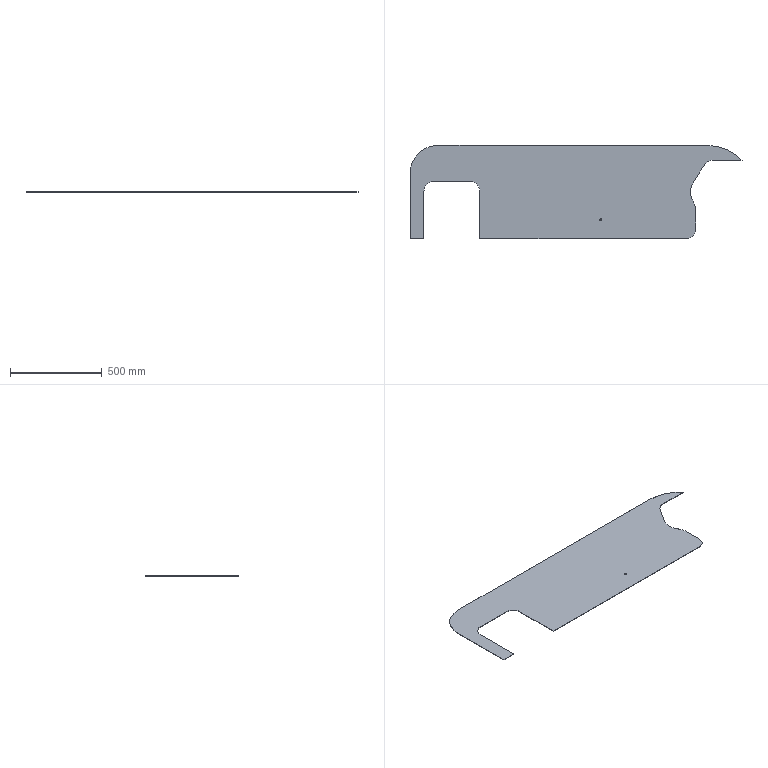Part | SolidWorks | features Extrusion 1 | 1 solid | 23 faces | box 1812 x 508 x 2 mm | volume 1419003 mm3 | plane 12 | cylinder 11 | commonest cylinder face diameters 101.6 x4 190.5 x3 11.176 x2 304.8 x1 508 x1
STEP:
#1=CARTESIAN_POINT('',(-589.788,-152.4,1.));
#2=VERTEX_POINT('',#1);
#3=CARTESIAN_POINT('',(-578.612,-152.4,1.));
#4=VERTEX_POINT('',#3);
#5=CARTESIAN_POINT('',(-584.2,-152.4,1.));
#6=DIRECTION('',(0.,0.,1.));
#7=DIRECTION('',(1.,0.,0.));
#8=AXIS2_PLACEMENT_3D('',#5,#6,#7);
#9=CIRCLE('',#8,5.588);
#10=EDGE_CURVE('',#2,#4,#9,.T.);
#11=ORIENTED_EDGE('',*,*,#10,.T.);
#12=CARTESIAN_POINT('',(-578.612,-152.4,-1.));
#13=VERTEX_POINT('',#12);
#14=CARTESIAN_POINT('',(-578.612,-152.4,1.));
#15=DIRECTION('',(0.,0.,-1.));
#16=VECTOR('',#15,1000.);
#17=LINE('',#14,#16);
#18=EDGE_CURVE('',#4,#13,#17,.T.);
#19=ORIENTED_EDGE('',*,*,#18,.T.);
#20=CARTESIAN_POINT('',(-589.788,-152.4,-1.));
#21=VERTEX_POINT('',#20);
#22=CARTESIAN_POINT('',(-584.2,-152.4,-1.));
#23=DIRECTION('',(0.,0.,1.));
#24=DIRECTION('',(1.,0.,0.));
#25=AXIS2_PLACEMENT_3D('',#22,#23,#24);
#26=CIRCLE('',#25,5.588);
#27=EDGE_CURVE('',#21,#13,#26,.T.);
#28=ORIENTED_EDGE('',*,*,#27,.F.);
#29=CARTESIAN_POINT('',(-589.788,-152.4,1.));
#30=DIRECTION('',(0.,0.,-1.));
#31=VECTOR('',#30,1000.);
#32=LINE('',#29,#31);
#33=EDGE_CURVE('',#2,#21,#32,.T.);
#34=ORIENTED_EDGE('',*,*,#33,.F.);
#35=EDGE_LOOP('',(#11,#19,#28,#34));
#36=FACE_OUTER_BOUND('',#35,.T.);
#37=CARTESIAN_POINT('',(-584.2,-152.4,1.));
#38=DIRECTION('',(0.,0.,-1.));
#39=DIRECTION('',(-1.,0.,0.));
#40=AXIS2_PLACEMENT_3D('',#37,#38,#39);
#41=CYLINDRICAL_SURFACE('',#40,5.588);
#42=ADVANCED_FACE('',(#36),#41,.F.);
#43=CARTESIAN_POINT('',(-95.25,0.,1.));
#44=VERTEX_POINT('',#43);
#45=CARTESIAN_POINT('',(-80.172,51.429,1.));
#46=VERTEX_POINT('',#45);
#47=CARTESIAN_POINT('',(0.,0.,1.));
#48=DIRECTION('',(0.,0.,-1.));
#49=DIRECTION('',(1.,0.,0.));
#50=AXIS2_PLACEMENT_3D('',#47,#48,#49);
#51=CIRCLE('',#50,95.25);
#52=EDGE_CURVE('',#44,#46,#51,.T.);
#53=ORIENTED_EDGE('',*,*,#52,.F.);
#54=CARTESIAN_POINT('',(-95.25,0.,-1.));
#55=VERTEX_POINT('',#54);
#56=CARTESIAN_POINT('',(-95.25,0.,1.));
#57=DIRECTION('',(0.,0.,-1.));
#58=VECTOR('',#57,1000.);
#59=LINE('',#56,#58);
#60=EDGE_CURVE('',#44,#55,#59,.T.);
#61=ORIENTED_EDGE('',*,*,#60,.T.);
#62=CARTESIAN_POINT('',(-80.172,51.429,-1.));
#63=VERTEX_POINT('',#62);
#64=CARTESIAN_POINT('',(0.,0.,-1.));
#65=DIRECTION('',(0.,0.,-1.));
#66=DIRECTION('',(1.,0.,0.));
#67=AXIS2_PLACEMENT_3D('',#64,#65,#66);
#68=CIRCLE('',#67,95.25);
#69=EDGE_CURVE('',#55,#63,#68,.T.);
#70=ORIENTED_EDGE('',*,*,#69,.T.);
#71=CARTESIAN_POINT('',(-80.172,51.429,1.));
#72=DIRECTION('',(0.,0.,-1.));
#73=VECTOR('',#72,1000.);
#74=LINE('',#71,#73);
#75=EDGE_CURVE('',#46,#63,#74,.T.);
#76=ORIENTED_EDGE('',*,*,#75,.F.);
#77=EDGE_LOOP('',(#53,#61,#70,#76));
#78=FACE_OUTER_BOUND('',#77,.T.);
#79=CARTESIAN_POINT('',(0.,0.,1.));
#80=DIRECTION('',(0.,0.,-1.));
#81=DIRECTION('',(-1.,0.,0.));
#82=AXIS2_PLACEMENT_3D('',#79,#80,#81);
#83=CYLINDRICAL_SURFACE('',#82,95.25);
#84=ADVANCED_FACE('',(#78),#83,.F.);
#85=CARTESIAN_POINT('',(-66.04,-101.37,1.));
#86=VERTEX_POINT('',#85);
#87=CARTESIAN_POINT('',(-80.645,-50.685,1.));
#88=VERTEX_POINT('',#87);
#89=CARTESIAN_POINT('',(-161.29,-101.37,1.));
#90=DIRECTION('',(0.,0.,1.));
#91=DIRECTION('',(1.,0.,0.));
#92=AXIS2_PLACEMENT_3D('',#89,#90,#91);
#93=CIRCLE('',#92,95.25);
#94=EDGE_CURVE('',#86,#88,#93,.T.);
#95=ORIENTED_EDGE('',*,*,#94,.T.);
#96=CARTESIAN_POINT('',(0.,0.,1.));
#97=DIRECTION('',(0.,0.,-1.));
#98=DIRECTION('',(1.,0.,0.));
#99=AXIS2_PLACEMENT_3D('',#96,#97,#98);
#100=CIRCLE('',#99,95.25);
#101=EDGE_CURVE('',#88,#44,#100,.T.);
#102=ORIENTED_EDGE('',*,*,#101,.T.);
#103=ORIENTED_EDGE('',*,*,#52,.T.);
#104=CARTESIAN_POINT('',(-17.359,149.349,1.));
#105=VERTEX_POINT('',#104);
#106=CARTESIAN_POINT('',(-17.359,149.349,1.));
#107=DIRECTION('',(0.5399,0.8417,0.));
#108=VECTOR('',#107,1000.);
#109=LINE('',#106,#108);
#110=EDGE_CURVE('',#46,#105,#109,.T.);
#111=ORIENTED_EDGE('',*,*,#110,.T.);
#112=CARTESIAN_POINT('',(25.4,172.72,1.));
#113=VERTEX_POINT('',#112);
#114=CARTESIAN_POINT('',(25.4,121.92,1.));
#115=DIRECTION('',(0.,0.,-1.));
#116=DIRECTION('',(1.,0.,0.));
#117=AXIS2_PLACEMENT_3D('',#114,#115,#116);
#118=CIRCLE('',#117,50.8);
#119=EDGE_CURVE('',#105,#113,#118,.T.);
#120=ORIENTED_EDGE('',*,*,#119,.T.);
#121=CARTESIAN_POINT('',(186.236,172.72,1.));
#122=VERTEX_POINT('',#121);
#123=CARTESIAN_POINT('',(186.236,172.72,1.));
#124=DIRECTION('',(1.,0.,0.));
#125=VECTOR('',#124,1000.);
#126=LINE('',#123,#125);
#127=EDGE_CURVE('',#113,#122,#126,.T.);
#128=ORIENTED_EDGE('',*,*,#127,.T.);
#129=CARTESIAN_POINT('',(0.,254.,1.));
#130=VERTEX_POINT('',#129);
#131=CARTESIAN_POINT('',(0.,0.,1.));
#132=DIRECTION('',(0.,0.,1.));
#133=DIRECTION('',(1.,0.,0.));
#134=AXIS2_PLACEMENT_3D('',#131,#132,#133);
#135=CIRCLE('',#134,254.);
#136=EDGE_CURVE('',#122,#130,#135,.T.);
#137=ORIENTED_EDGE('',*,*,#136,.T.);
#138=CARTESIAN_POINT('',(-1473.2,254.,1.));
#139=VERTEX_POINT('',#138);
#140=CARTESIAN_POINT('',(0.,254.,1.));
#141=DIRECTION('',(-1.,0.,0.));
#142=VECTOR('',#141,1000.);
#143=LINE('',#140,#142);
#144=EDGE_CURVE('',#130,#139,#143,.T.);
#145=ORIENTED_EDGE('',*,*,#144,.T.);
#146=CARTESIAN_POINT('',(-1625.6,101.6,1.));
#147=VERTEX_POINT('',#146);
#148=CARTESIAN_POINT('',(-1473.2,101.6,1.));
#149=DIRECTION('',(0.,0.,1.));
#150=DIRECTION('',(1.,0.,0.));
#151=AXIS2_PLACEMENT_3D('',#148,#149,#150);
#152=CIRCLE('',#151,152.4);
#153=EDGE_CURVE('',#139,#147,#152,.T.);
#154=ORIENTED_EDGE('',*,*,#153,.T.);
#155=CARTESIAN_POINT('',(-1625.6,-254.,1.));
#156=VERTEX_POINT('',#155);
#157=CARTESIAN_POINT('',(-1625.6,101.6,1.));
#158=DIRECTION('',(0.,-1.,0.));
#159=VECTOR('',#158,1000.);
#160=LINE('',#157,#159);
#161=EDGE_CURVE('',#147,#156,#160,.T.);
#162=ORIENTED_EDGE('',*,*,#161,.T.);
#163=CARTESIAN_POINT('',(-1549.4,-254.,1.));
#164=VERTEX_POINT('',#163);
#165=CARTESIAN_POINT('',(-1549.4,-254.,1.));
#166=DIRECTION('',(1.,0.,0.));
#167=VECTOR('',#166,1000.);
#168=LINE('',#165,#167);
#169=EDGE_CURVE('',#156,#164,#168,.T.);
#170=ORIENTED_EDGE('',*,*,#169,.T.);
#171=CARTESIAN_POINT('',(-1549.4,5.08,1.));
#172=VERTEX_POINT('',#171);
#173=CARTESIAN_POINT('',(-1549.4,-254.,1.));
#174=DIRECTION('',(0.,1.,0.));
#175=VECTOR('',#174,1000.);
#176=LINE('',#173,#175);
#177=EDGE_CURVE('',#164,#172,#176,.T.);
#178=ORIENTED_EDGE('',*,*,#177,.T.);
#179=CARTESIAN_POINT('',(-1498.6,55.88,1.));
#180=VERTEX_POINT('',#179);
#181=CARTESIAN_POINT('',(-1498.6,5.08,1.));
#182=DIRECTION('',(0.,0.,-1.));
#183=DIRECTION('',(-1.,0.,0.));
#184=AXIS2_PLACEMENT_3D('',#181,#182,#183);
#185=CIRCLE('',#184,50.8);
#186=EDGE_CURVE('',#172,#180,#185,.T.);
#187=ORIENTED_EDGE('',*,*,#186,.T.);
#188=CARTESIAN_POINT('',(-1295.4,55.88,1.));
#189=VERTEX_POINT('',#188);
#190=CARTESIAN_POINT('',(-1498.6,55.88,1.));
#191=DIRECTION('',(1.,0.,0.));
#192=VECTOR('',#191,1000.);
#193=LINE('',#190,#192);
#194=EDGE_CURVE('',#180,#189,#193,.T.);
#195=ORIENTED_EDGE('',*,*,#194,.T.);
#196=CARTESIAN_POINT('',(-1244.6,5.08,1.));
#197=VERTEX_POINT('',#196);
#198=CARTESIAN_POINT('',(-1295.4,5.08,1.));
#199=DIRECTION('',(0.,0.,-1.));
#200=DIRECTION('',(-1.,0.,0.));
#201=AXIS2_PLACEMENT_3D('',#198,#199,#200);
#202=CIRCLE('',#201,50.8);
#203=EDGE_CURVE('',#189,#197,#202,.T.);
#204=ORIENTED_EDGE('',*,*,#203,.T.);
#205=CARTESIAN_POINT('',(-1244.6,-254.,1.));
#206=VERTEX_POINT('',#205);
#207=CARTESIAN_POINT('',(-1244.6,5.08,1.));
#208=DIRECTION('',(0.,-1.,0.));
#209=VECTOR('',#208,1000.);
#210=LINE('',#207,#209);
#211=EDGE_CURVE('',#197,#206,#210,.T.);
#212=ORIENTED_EDGE('',*,*,#211,.T.);
#213=CARTESIAN_POINT('',(-116.84,-254.,1.));
#214=VERTEX_POINT('',#213);
#215=CARTESIAN_POINT('',(-116.84,-254.,1.));
#216=DIRECTION('',(1.,0.,0.));
#217=VECTOR('',#216,1000.);
#218=LINE('',#215,#217);
#219=EDGE_CURVE('',#206,#214,#218,.T.);
#220=ORIENTED_EDGE('',*,*,#219,.T.);
#221=CARTESIAN_POINT('',(-66.04,-203.2,1.));
#222=VERTEX_POINT('',#221);
#223=CARTESIAN_POINT('',(-116.84,-203.2,1.));
#224=DIRECTION('',(0.,0.,1.));
#225=DIRECTION('',(-1.,0.,0.));
#226=AXIS2_PLACEMENT_3D('',#223,#224,#225);
#227=CIRCLE('',#226,50.8);
#228=EDGE_CURVE('',#214,#222,#227,.T.);
#229=ORIENTED_EDGE('',*,*,#228,.T.);
#230=CARTESIAN_POINT('',(-66.04,-101.37,1.));
#231=DIRECTION('',(0.,1.,0.));
#232=VECTOR('',#231,1000.);
#233=LINE('',#230,#232);
#234=EDGE_CURVE('',#222,#86,#233,.T.);
#235=ORIENTED_EDGE('',*,*,#234,.T.);
#236=EDGE_LOOP('',(#95,#102,#103,#111,#120,#128,#137,#145,#154,#162,#170,#178,#187,#195,#204,#212,#220,#229,#235));
#237=FACE_OUTER_BOUND('',#236,.T.);
#238=ORIENTED_EDGE('',*,*,#10,.F.);
#239=CARTESIAN_POINT('',(-584.2,-152.4,1.));
#240=DIRECTION('',(0.,0.,1.));
#241=DIRECTION('',(1.,0.,0.));
#242=AXIS2_PLACEMENT_3D('',#239,#240,#241);
#243=CIRCLE('',#242,5.588);
#244=EDGE_CURVE('',#4,#2,#243,.T.);
#245=ORIENTED_EDGE('',*,*,#244,.F.);
#246=EDGE_LOOP('',(#238,#245));
#247=FACE_BOUND('',#246,.T.);
#248=CARTESIAN_POINT('',(-161.29,-101.37,1.));
#249=DIRECTION('',(0.,0.,1.));
#250=DIRECTION('',(1.,0.,0.));
#251=AXIS2_PLACEMENT_3D('',#248,#249,#250);
#252=PLANE('',#251);
#253=ADVANCED_FACE('',(#237,#247),#252,.T.);
#254=CARTESIAN_POINT('',(-66.04,-101.37,-1.));
#255=VERTEX_POINT('',#254);
#256=CARTESIAN_POINT('',(-80.645,-50.685,-1.));
#257=VERTEX_POINT('',#256);
#258=CARTESIAN_POINT('',(-161.29,-101.37,-1.));
#259=DIRECTION('',(0.,0.,1.));
#260=DIRECTION('',(1.,0.,0.));
#261=AXIS2_PLACEMENT_3D('',#258,#259,#260);
#262=CIRCLE('',#261,95.25);
#263=EDGE_CURVE('',#255,#257,#262,.T.);
#264=ORIENTED_EDGE('',*,*,#263,.F.);
#265=CARTESIAN_POINT('',(-66.04,-203.2,-1.));
#266=VERTEX_POINT('',#265);
#267=CARTESIAN_POINT('',(-66.04,-101.37,-1.));
#268=DIRECTION('',(0.,1.,0.));
#269=VECTOR('',#268,1000.);
#270=LINE('',#267,#269);
#271=EDGE_CURVE('',#266,#255,#270,.T.);
#272=ORIENTED_EDGE('',*,*,#271,.F.);
#273=CARTESIAN_POINT('',(-116.84,-254.,-1.));
#274=VERTEX_POINT('',#273);
#275=CARTESIAN_POINT('',(-116.84,-203.2,-1.));
#276=DIRECTION('',(0.,0.,1.));
#277=DIRECTION('',(-1.,0.,0.));
#278=AXIS2_PLACEMENT_3D('',#275,#276,#277);
#279=CIRCLE('',#278,50.8);
#280=EDGE_CURVE('',#274,#266,#279,.T.);
#281=ORIENTED_EDGE('',*,*,#280,.F.);
#282=CARTESIAN_POINT('',(-1244.6,-254.,-1.));
#283=VERTEX_POINT('',#282);
#284=CARTESIAN_POINT('',(-116.84,-254.,-1.));
#285=DIRECTION('',(1.,0.,0.));
#286=VECTOR('',#285,1000.);
#287=LINE('',#284,#286);
#288=EDGE_CURVE('',#283,#274,#287,.T.);
#289=ORIENTED_EDGE('',*,*,#288,.F.);
#290=CARTESIAN_POINT('',(-1244.6,5.08,-1.));
#291=VERTEX_POINT('',#290);
#292=CARTESIAN_POINT('',(-1244.6,5.08,-1.));
#293=DIRECTION('',(0.,-1.,0.));
#294=VECTOR('',#293,1000.);
#295=LINE('',#292,#294);
#296=EDGE_CURVE('',#291,#283,#295,.T.);
#297=ORIENTED_EDGE('',*,*,#296,.F.);
#298=CARTESIAN_POINT('',(-1295.4,55.88,-1.));
#299=VERTEX_POINT('',#298);
#300=CARTESIAN_POINT('',(-1295.4,5.08,-1.));
#301=DIRECTION('',(0.,0.,-1.));
#302=DIRECTION('',(-1.,0.,0.));
#303=AXIS2_PLACEMENT_3D('',#300,#301,#302);
#304=CIRCLE('',#303,50.8);
#305=EDGE_CURVE('',#299,#291,#304,.T.);
#306=ORIENTED_EDGE('',*,*,#305,.F.);
#307=CARTESIAN_POINT('',(-1498.6,55.88,-1.));
#308=VERTEX_POINT('',#307);
#309=CARTESIAN_POINT('',(-1498.6,55.88,-1.));
#310=DIRECTION('',(1.,0.,0.));
#311=VECTOR('',#310,1000.);
#312=LINE('',#309,#311);
#313=EDGE_CURVE('',#308,#299,#312,.T.);
#314=ORIENTED_EDGE('',*,*,#313,.F.);
#315=CARTESIAN_POINT('',(-1549.4,5.08,-1.));
#316=VERTEX_POINT('',#315);
#317=CARTESIAN_POINT('',(-1498.6,5.08,-1.));
#318=DIRECTION('',(0.,0.,-1.));
#319=DIRECTION('',(-1.,0.,0.));
#320=AXIS2_PLACEMENT_3D('',#317,#318,#319);
#321=CIRCLE('',#320,50.8);
#322=EDGE_CURVE('',#316,#308,#321,.T.);
#323=ORIENTED_EDGE('',*,*,#322,.F.);
#324=CARTESIAN_POINT('',(-1549.4,-254.,-1.));
#325=VERTEX_POINT('',#324);
#326=CARTESIAN_POINT('',(-1549.4,-254.,-1.));
#327=DIRECTION('',(0.,1.,0.));
#328=VECTOR('',#327,1000.);
#329=LINE('',#326,#328);
#330=EDGE_CURVE('',#325,#316,#329,.T.);
#331=ORIENTED_EDGE('',*,*,#330,.F.);
#332=CARTESIAN_POINT('',(-1625.6,-254.,-1.));
#333=VERTEX_POINT('',#332);
#334=CARTESIAN_POINT('',(-1549.4,-254.,-1.));
#335=DIRECTION('',(1.,0.,0.));
#336=VECTOR('',#335,1000.);
#337=LINE('',#334,#336);
#338=EDGE_CURVE('',#333,#325,#337,.T.);
#339=ORIENTED_EDGE('',*,*,#338,.F.);
#340=CARTESIAN_POINT('',(-1625.6,101.6,-1.));
#341=VERTEX_POINT('',#340);
#342=CARTESIAN_POINT('',(-1625.6,101.6,-1.));
#343=DIRECTION('',(0.,-1.,0.));
#344=VECTOR('',#343,1000.);
#345=LINE('',#342,#344);
#346=EDGE_CURVE('',#341,#333,#345,.T.);
#347=ORIENTED_EDGE('',*,*,#346,.F.);
#348=CARTESIAN_POINT('',(-1473.2,254.,-1.));
#349=VERTEX_POINT('',#348);
#350=CARTESIAN_POINT('',(-1473.2,101.6,-1.));
#351=DIRECTION('',(0.,0.,1.));
#352=DIRECTION('',(1.,0.,0.));
#353=AXIS2_PLACEMENT_3D('',#350,#351,#352);
#354=CIRCLE('',#353,152.4);
#355=EDGE_CURVE('',#349,#341,#354,.T.);
#356=ORIENTED_EDGE('',*,*,#355,.F.);
#357=CARTESIAN_POINT('',(0.,254.,-1.));
#358=VERTEX_POINT('',#357);
#359=CARTESIAN_POINT('',(0.,254.,-1.));
#360=DIRECTION('',(-1.,0.,0.));
#361=VECTOR('',#360,1000.);
#362=LINE('',#359,#361);
#363=EDGE_CURVE('',#358,#349,#362,.T.);
#364=ORIENTED_EDGE('',*,*,#363,.F.);
#365=CARTESIAN_POINT('',(186.236,172.72,-1.));
#366=VERTEX_POINT('',#365);
#367=CARTESIAN_POINT('',(0.,0.,-1.));
#368=DIRECTION('',(0.,0.,1.));
#369=DIRECTION('',(1.,0.,0.));
#370=AXIS2_PLACEMENT_3D('',#367,#368,#369);
#371=CIRCLE('',#370,254.);
#372=EDGE_CURVE('',#366,#358,#371,.T.);
#373=ORIENTED_EDGE('',*,*,#372,.F.);
#374=CARTESIAN_POINT('',(25.4,172.72,-1.));
#375=VERTEX_POINT('',#374);
#376=CARTESIAN_POINT('',(186.236,172.72,-1.));
#377=DIRECTION('',(1.,0.,0.));
#378=VECTOR('',#377,1000.);
#379=LINE('',#376,#378);
#380=EDGE_CURVE('',#375,#366,#379,.T.);
#381=ORIENTED_EDGE('',*,*,#380,.F.);
#382=CARTESIAN_POINT('',(-17.359,149.349,-1.));
#383=VERTEX_POINT('',#382);
#384=CARTESIAN_POINT('',(25.4,121.92,-1.));
#385=DIRECTION('',(0.,0.,-1.));
#386=DIRECTION('',(1.,0.,0.));
#387=AXIS2_PLACEMENT_3D('',#384,#385,#386);
#388=CIRCLE('',#387,50.8);
#389=EDGE_CURVE('',#383,#375,#388,.T.);
#390=ORIENTED_EDGE('',*,*,#389,.F.);
#391=CARTESIAN_POINT('',(-17.359,149.349,-1.));
#392=DIRECTION('',(0.5399,0.8417,0.));
#393=VECTOR('',#392,1000.);
#394=LINE('',#391,#393);
#395=EDGE_CURVE('',#63,#383,#394,.T.);
#396=ORIENTED_EDGE('',*,*,#395,.F.);
#397=ORIENTED_EDGE('',*,*,#69,.F.);
#398=CARTESIAN_POINT('',(0.,0.,-1.));
#399=DIRECTION('',(0.,0.,-1.));
#400=DIRECTION('',(1.,0.,0.));
#401=AXIS2_PLACEMENT_3D('',#398,#399,#400);
#402=CIRCLE('',#401,95.25);
#403=EDGE_CURVE('',#257,#55,#402,.T.);
#404=ORIENTED_EDGE('',*,*,#403,.F.);
#405=EDGE_LOOP('',(#264,#272,#281,#289,#297,#306,#314,#323,#331,#339,#347,#356,#364,#373,#381,#390,#396,#397,#404));
#406=FACE_OUTER_BOUND('',#405,.T.);
#407=ORIENTED_EDGE('',*,*,#27,.T.);
#408=CARTESIAN_POINT('',(-584.2,-152.4,-1.));
#409=DIRECTION('',(0.,0.,1.));
#410=DIRECTION('',(1.,0.,0.));
#411=AXIS2_PLACEMENT_3D('',#408,#409,#410);
#412=CIRCLE('',#411,5.588);
#413=EDGE_CURVE('',#13,#21,#412,.T.);
#414=ORIENTED_EDGE('',*,*,#413,.T.);
#415=EDGE_LOOP('',(#407,#414));
#416=FACE_BOUND('',#415,.T.);
#417=CARTESIAN_POINT('',(-161.29,-101.37,-1.));
#418=DIRECTION('',(0.,0.,1.));
#419=DIRECTION('',(1.,0.,0.));
#420=AXIS2_PLACEMENT_3D('',#417,#418,#419);
#421=PLANE('',#420);
#422=ADVANCED_FACE('',(#406,#416),#421,.F.);
#423=ORIENTED_EDGE('',*,*,#263,.T.);
#424=CARTESIAN_POINT('',(-80.645,-50.685,1.));
#425=DIRECTION('',(0.,0.,-1.));
#426=VECTOR('',#425,1000.);
#427=LINE('',#424,#426);
#428=EDGE_CURVE('',#88,#257,#427,.T.);
#429=ORIENTED_EDGE('',*,*,#428,.F.);
#430=ORIENTED_EDGE('',*,*,#94,.F.);
#431=CARTESIAN_POINT('',(-66.04,-101.37,1.));
#432=DIRECTION('',(0.,0.,-1.));
#433=VECTOR('',#432,1000.);
#434=LINE('',#431,#433);
#435=EDGE_CURVE('',#86,#255,#434,.T.);
#436=ORIENTED_EDGE('',*,*,#435,.T.);
#437=EDGE_LOOP('',(#423,#429,#430,#436));
#438=FACE_OUTER_BOUND('',#437,.T.);
#439=CARTESIAN_POINT('',(-161.29,-101.37,1.));
#440=DIRECTION('',(0.,0.,-1.));
#441=DIRECTION('',(-1.,0.,0.));
#442=AXIS2_PLACEMENT_3D('',#439,#440,#441);
#443=CYLINDRICAL_SURFACE('',#442,95.25);
#444=ADVANCED_FACE('',(#438),#443,.T.);
#445=ORIENTED_EDGE('',*,*,#60,.F.);
#446=ORIENTED_EDGE('',*,*,#101,.F.);
#447=ORIENTED_EDGE('',*,*,#428,.T.);
#448=ORIENTED_EDGE('',*,*,#403,.T.);
#449=EDGE_LOOP('',(#445,#446,#447,#448));
#450=FACE_OUTER_BOUND('',#449,.T.);
#451=CARTESIAN_POINT('',(0.,0.,1.));
#452=DIRECTION('',(0.,0.,-1.));
#453=DIRECTION('',(-1.,0.,0.));
#454=AXIS2_PLACEMENT_3D('',#451,#452,#453);
#455=CYLINDRICAL_SURFACE('',#454,95.25);
#456=ADVANCED_FACE('',(#450),#455,.F.);
#457=ORIENTED_EDGE('',*,*,#395,.T.);
#458=CARTESIAN_POINT('',(-17.359,149.349,1.));
#459=DIRECTION('',(0.,0.,-1.));
#460=VECTOR('',#459,1000.);
#461=LINE('',#458,#460);
#462=EDGE_CURVE('',#105,#383,#461,.T.);
#463=ORIENTED_EDGE('',*,*,#462,.F.);
#464=ORIENTED_EDGE('',*,*,#110,.F.);
#465=ORIENTED_EDGE('',*,*,#75,.T.);
#466=EDGE_LOOP('',(#457,#463,#464,#465));
#467=FACE_OUTER_BOUND('',#466,.T.);
#468=CARTESIAN_POINT('',(-17.359,149.349,1.));
#469=DIRECTION('',(-0.8417,0.5399,0.));
#470=DIRECTION('',(-0.5399,-0.8417,0.));
#471=AXIS2_PLACEMENT_3D('',#468,#469,#470);
#472=PLANE('',#471);
#473=ADVANCED_FACE('',(#467),#472,.F.);
#474=ORIENTED_EDGE('',*,*,#389,.T.);
#475=CARTESIAN_POINT('',(25.4,172.72,1.));
#476=DIRECTION('',(0.,0.,-1.));
#477=VECTOR('',#476,1000.);
#478=LINE('',#475,#477);
#479=EDGE_CURVE('',#113,#375,#478,.T.);
#480=ORIENTED_EDGE('',*,*,#479,.F.);
#481=ORIENTED_EDGE('',*,*,#119,.F.);
#482=ORIENTED_EDGE('',*,*,#462,.T.);
#483=EDGE_LOOP('',(#474,#480,#481,#482));
#484=FACE_OUTER_BOUND('',#483,.T.);
#485=CARTESIAN_POINT('',(25.4,121.92,1.));
#486=DIRECTION('',(0.,0.,-1.));
#487=DIRECTION('',(-1.,0.,0.));
#488=AXIS2_PLACEMENT_3D('',#485,#486,#487);
#489=CYLINDRICAL_SURFACE('',#488,50.8);
#490=ADVANCED_FACE('',(#484),#489,.F.);
#491=ORIENTED_EDGE('',*,*,#380,.T.);
#492=CARTESIAN_POINT('',(186.236,172.72,1.));
#493=DIRECTION('',(0.,0.,-1.));
#494=VECTOR('',#493,1000.);
#495=LINE('',#492,#494);
#496=EDGE_CURVE('',#122,#366,#495,.T.);
#497=ORIENTED_EDGE('',*,*,#496,.F.);
#498=ORIENTED_EDGE('',*,*,#127,.F.);
#499=ORIENTED_EDGE('',*,*,#479,.T.);
#500=EDGE_LOOP('',(#491,#497,#498,#499));
#501=FACE_OUTER_BOUND('',#500,.T.);
#502=CARTESIAN_POINT('',(186.236,172.72,1.));
#503=DIRECTION('',(0.,1.,0.));
#504=DIRECTION('',(-1.,0.,0.));
#505=AXIS2_PLACEMENT_3D('',#502,#503,#504);
#506=PLANE('',#505);
#507=ADVANCED_FACE('',(#501),#506,.F.);
#508=ORIENTED_EDGE('',*,*,#372,.T.);
#509=CARTESIAN_POINT('',(0.,254.,1.));
#510=DIRECTION('',(0.,0.,-1.));
#511=VECTOR('',#510,1000.);
#512=LINE('',#509,#511);
#513=EDGE_CURVE('',#130,#358,#512,.T.);
#514=ORIENTED_EDGE('',*,*,#513,.F.);
#515=ORIENTED_EDGE('',*,*,#136,.F.);
#516=ORIENTED_EDGE('',*,*,#496,.T.);
#517=EDGE_LOOP('',(#508,#514,#515,#516));
#518=FACE_OUTER_BOUND('',#517,.T.);
#519=CARTESIAN_POINT('',(0.,0.,1.));
#520=DIRECTION('',(0.,0.,-1.));
#521=DIRECTION('',(-1.,0.,0.));
#522=AXIS2_PLACEMENT_3D('',#519,#520,#521);
#523=CYLINDRICAL_SURFACE('',#522,254.);
#524=ADVANCED_FACE('',(#518),#523,.T.);
#525=ORIENTED_EDGE('',*,*,#363,.T.);
#526=CARTESIAN_POINT('',(-1473.2,254.,1.));
#527=DIRECTION('',(0.,0.,-1.));
#528=VECTOR('',#527,1000.);
#529=LINE('',#526,#528);
#530=EDGE_CURVE('',#139,#349,#529,.T.);
#531=ORIENTED_EDGE('',*,*,#530,.F.);
#532=ORIENTED_EDGE('',*,*,#144,.F.);
#533=ORIENTED_EDGE('',*,*,#513,.T.);
#534=EDGE_LOOP('',(#525,#531,#532,#533));
#535=FACE_OUTER_BOUND('',#534,.T.);
#536=CARTESIAN_POINT('',(0.,254.,1.));
#537=DIRECTION('',(0.,-1.,0.));
#538=DIRECTION('',(1.,0.,0.));
#539=AXIS2_PLACEMENT_3D('',#536,#537,#538);
#540=PLANE('',#539);
#541=ADVANCED_FACE('',(#535),#540,.F.);
#542=ORIENTED_EDGE('',*,*,#355,.T.);
#543=CARTESIAN_POINT('',(-1625.6,101.6,1.));
#544=DIRECTION('',(0.,0.,-1.));
#545=VECTOR('',#544,1000.);
#546=LINE('',#543,#545);
#547=EDGE_CURVE('',#147,#341,#546,.T.);
#548=ORIENTED_EDGE('',*,*,#547,.F.);
#549=ORIENTED_EDGE('',*,*,#153,.F.);
#550=ORIENTED_EDGE('',*,*,#530,.T.);
#551=EDGE_LOOP('',(#542,#548,#549,#550));
#552=FACE_OUTER_BOUND('',#551,.T.);
#553=CARTESIAN_POINT('',(-1473.2,101.6,1.));
#554=DIRECTION('',(0.,0.,-1.));
#555=DIRECTION('',(-1.,0.,0.));
#556=AXIS2_PLACEMENT_3D('',#553,#554,#555);
#557=CYLINDRICAL_SURFACE('',#556,152.4);
#558=ADVANCED_FACE('',(#552),#557,.T.);
#559=ORIENTED_EDGE('',*,*,#346,.T.);
#560=CARTESIAN_POINT('',(-1625.6,-254.,1.));
#561=DIRECTION('',(0.,0.,-1.));
#562=VECTOR('',#561,1000.);
#563=LINE('',#560,#562);
#564=EDGE_CURVE('',#156,#333,#563,.T.);
#565=ORIENTED_EDGE('',*,*,#564,.F.);
#566=ORIENTED_EDGE('',*,*,#161,.F.);
#567=ORIENTED_EDGE('',*,*,#547,.T.);
#568=EDGE_LOOP('',(#559,#565,#566,#567));
#569=FACE_OUTER_BOUND('',#568,.T.);
#570=CARTESIAN_POINT('',(-1625.6,101.6,1.));
#571=DIRECTION('',(1.,0.,0.));
#572=DIRECTION('',(0.,0.,-1.));
#573=AXIS2_PLACEMENT_3D('',#570,#571,#572);
#574=PLANE('',#573);
#575=ADVANCED_FACE('',(#569),#574,.F.);
#576=ORIENTED_EDGE('',*,*,#338,.T.);
#577=CARTESIAN_POINT('',(-1549.4,-254.,1.));
#578=DIRECTION('',(0.,0.,-1.));
#579=VECTOR('',#578,1000.);
#580=LINE('',#577,#579);
#581=EDGE_CURVE('',#164,#325,#580,.T.);
#582=ORIENTED_EDGE('',*,*,#581,.F.);
#583=ORIENTED_EDGE('',*,*,#169,.F.);
#584=ORIENTED_EDGE('',*,*,#564,.T.);
#585=EDGE_LOOP('',(#576,#582,#583,#584));
#586=FACE_OUTER_BOUND('',#585,.T.);
#587=CARTESIAN_POINT('',(-1549.4,-254.,1.));
#588=DIRECTION('',(0.,1.,0.));
#589=DIRECTION('',(-1.,0.,0.));
#590=AXIS2_PLACEMENT_3D('',#587,#588,#589);
#591=PLANE('',#590);
#592=ADVANCED_FACE('',(#586),#591,.F.);
#593=ORIENTED_EDGE('',*,*,#330,.T.);
#594=CARTESIAN_POINT('',(-1549.4,5.08,1.));
#595=DIRECTION('',(0.,0.,-1.));
#596=VECTOR('',#595,1000.);
#597=LINE('',#594,#596);
#598=EDGE_CURVE('',#172,#316,#597,.T.);
#599=ORIENTED_EDGE('',*,*,#598,.F.);
#600=ORIENTED_EDGE('',*,*,#177,.F.);
#601=ORIENTED_EDGE('',*,*,#581,.T.);
#602=EDGE_LOOP('',(#593,#599,#600,#601));
#603=FACE_OUTER_BOUND('',#602,.T.);
#604=CARTESIAN_POINT('',(-1549.4,-254.,1.));
#605=DIRECTION('',(-1.,0.,0.));
#606=DIRECTION('',(0.,0.,1.));
#607=AXIS2_PLACEMENT_3D('',#604,#605,#606);
#608=PLANE('',#607);
#609=ADVANCED_FACE('',(#603),#608,.F.);
#610=ORIENTED_EDGE('',*,*,#322,.T.);
#611=CARTESIAN_POINT('',(-1498.6,55.88,1.));
#612=DIRECTION('',(0.,0.,-1.));
#613=VECTOR('',#612,1000.);
#614=LINE('',#611,#613);
#615=EDGE_CURVE('',#180,#308,#614,.T.);
#616=ORIENTED_EDGE('',*,*,#615,.F.);
#617=ORIENTED_EDGE('',*,*,#186,.F.);
#618=ORIENTED_EDGE('',*,*,#598,.T.);
#619=EDGE_LOOP('',(#610,#616,#617,#618));
#620=FACE_OUTER_BOUND('',#619,.T.);
#621=CARTESIAN_POINT('',(-1498.6,5.08,1.));
#622=DIRECTION('',(0.,0.,-1.));
#623=DIRECTION('',(-1.,0.,0.));
#624=AXIS2_PLACEMENT_3D('',#621,#622,#623);
#625=CYLINDRICAL_SURFACE('',#624,50.8);
#626=ADVANCED_FACE('',(#620),#625,.F.);
#627=ORIENTED_EDGE('',*,*,#313,.T.);
#628=CARTESIAN_POINT('',(-1295.4,55.88,1.));
#629=DIRECTION('',(0.,0.,-1.));
#630=VECTOR('',#629,1000.);
#631=LINE('',#628,#630);
#632=EDGE_CURVE('',#189,#299,#631,.T.);
#633=ORIENTED_EDGE('',*,*,#632,.F.);
#634=ORIENTED_EDGE('',*,*,#194,.F.);
#635=ORIENTED_EDGE('',*,*,#615,.T.);
#636=EDGE_LOOP('',(#627,#633,#634,#635));
#637=FACE_OUTER_BOUND('',#636,.T.);
#638=CARTESIAN_POINT('',(-1498.6,55.88,1.));
#639=DIRECTION('',(0.,1.,0.));
#640=DIRECTION('',(0.,0.,1.));
#641=AXIS2_PLACEMENT_3D('',#638,#639,#640);
#642=PLANE('',#641);
#643=ADVANCED_FACE('',(#637),#642,.F.);
#644=ORIENTED_EDGE('',*,*,#305,.T.);
#645=CARTESIAN_POINT('',(-1244.6,5.08,1.));
#646=DIRECTION('',(0.,0.,-1.));
#647=VECTOR('',#646,1000.);
#648=LINE('',#645,#647);
#649=EDGE_CURVE('',#197,#291,#648,.T.);
#650=ORIENTED_EDGE('',*,*,#649,.F.);
#651=ORIENTED_EDGE('',*,*,#203,.F.);
#652=ORIENTED_EDGE('',*,*,#632,.T.);
#653=EDGE_LOOP('',(#644,#650,#651,#652));
#654=FACE_OUTER_BOUND('',#653,.T.);
#655=CARTESIAN_POINT('',(-1295.4,5.08,1.));
#656=DIRECTION('',(0.,0.,-1.));
#657=DIRECTION('',(-1.,0.,0.));
#658=AXIS2_PLACEMENT_3D('',#655,#656,#657);
#659=CYLINDRICAL_SURFACE('',#658,50.8);
#660=ADVANCED_FACE('',(#654),#659,.F.);
#661=ORIENTED_EDGE('',*,*,#296,.T.);
#662=CARTESIAN_POINT('',(-1244.6,-254.,1.));
#663=DIRECTION('',(0.,0.,-1.));
#664=VECTOR('',#663,1000.);
#665=LINE('',#662,#664);
#666=EDGE_CURVE('',#206,#283,#665,.T.);
#667=ORIENTED_EDGE('',*,*,#666,.F.);
#668=ORIENTED_EDGE('',*,*,#211,.F.);
#669=ORIENTED_EDGE('',*,*,#649,.T.);
#670=EDGE_LOOP('',(#661,#667,#668,#669));
#671=FACE_OUTER_BOUND('',#670,.T.);
#672=CARTESIAN_POINT('',(-1244.6,5.08,1.));
#673=DIRECTION('',(1.,0.,0.));
#674=DIRECTION('',(0.,0.,-1.));
#675=AXIS2_PLACEMENT_3D('',#672,#673,#674);
#676=PLANE('',#675);
#677=ADVANCED_FACE('',(#671),#676,.F.);
#678=ORIENTED_EDGE('',*,*,#288,.T.);
#679=CARTESIAN_POINT('',(-116.84,-254.,1.));
#680=DIRECTION('',(0.,0.,-1.));
#681=VECTOR('',#680,1000.);
#682=LINE('',#679,#681);
#683=EDGE_CURVE('',#214,#274,#682,.T.);
#684=ORIENTED_EDGE('',*,*,#683,.F.);
#685=ORIENTED_EDGE('',*,*,#219,.F.);
#686=ORIENTED_EDGE('',*,*,#666,.T.);
#687=EDGE_LOOP('',(#678,#684,#685,#686));
#688=FACE_OUTER_BOUND('',#687,.T.);
#689=CARTESIAN_POINT('',(-116.84,-254.,1.));
#690=DIRECTION('',(0.,1.,0.));
#691=DIRECTION('',(-1.,0.,0.));
#692=AXIS2_PLACEMENT_3D('',#689,#690,#691);
#693=PLANE('',#692);
#694=ADVANCED_FACE('',(#688),#693,.F.);
#695=ORIENTED_EDGE('',*,*,#280,.T.);
#696=CARTESIAN_POINT('',(-66.04,-203.2,1.));
#697=DIRECTION('',(0.,0.,-1.));
#698=VECTOR('',#697,1000.);
#699=LINE('',#696,#698);
#700=EDGE_CURVE('',#222,#266,#699,.T.);
#701=ORIENTED_EDGE('',*,*,#700,.F.);
#702=ORIENTED_EDGE('',*,*,#228,.F.);
#703=ORIENTED_EDGE('',*,*,#683,.T.);
#704=EDGE_LOOP('',(#695,#701,#702,#703));
#705=FACE_OUTER_BOUND('',#704,.T.);
#706=CARTESIAN_POINT('',(-116.84,-203.2,1.));
#707=DIRECTION('',(0.,0.,-1.));
#708=DIRECTION('',(-1.,0.,0.));
#709=AXIS2_PLACEMENT_3D('',#706,#707,#708);
#710=CYLINDRICAL_SURFACE('',#709,50.8);
#711=ADVANCED_FACE('',(#705),#710,.T.);
#712=ORIENTED_EDGE('',*,*,#271,.T.);
#713=ORIENTED_EDGE('',*,*,#435,.F.);
#714=ORIENTED_EDGE('',*,*,#234,.F.);
#715=ORIENTED_EDGE('',*,*,#700,.T.);
#716=EDGE_LOOP('',(#712,#713,#714,#715));
#717=FACE_OUTER_BOUND('',#716,.T.);
#718=CARTESIAN_POINT('',(-66.04,-101.37,1.));
#719=DIRECTION('',(-1.,0.,0.));
#720=DIRECTION('',(0.,-1.,0.));
#721=AXIS2_PLACEMENT_3D('',#718,#719,#720);
#722=PLANE('',#721);
#723=ADVANCED_FACE('',(#717),#722,.F.);
#724=ORIENTED_EDGE('',*,*,#18,.F.);
#725=ORIENTED_EDGE('',*,*,#244,.T.);
#726=ORIENTED_EDGE('',*,*,#33,.T.);
#727=ORIENTED_EDGE('',*,*,#413,.F.);
#728=EDGE_LOOP('',(#724,#725,#726,#727));
#729=FACE_OUTER_BOUND('',#728,.T.);
#730=CARTESIAN_POINT('',(-584.2,-152.4,1.));
#731=DIRECTION('',(0.,0.,-1.));
#732=DIRECTION('',(-1.,0.,0.));
#733=AXIS2_PLACEMENT_3D('',#730,#731,#732);
#734=CYLINDRICAL_SURFACE('',#733,5.588);
#735=ADVANCED_FACE('',(#729),#734,.F.);
#736=CLOSED_SHELL('',(#42,#84,#253,#422,#444,#456,#473,#490,#507,#524,#541,#558,#575,#592,#609,#626,#643,#660,#677,#694,#711,#723,#735));
#737=MANIFOLD_SOLID_BREP('',#736);
#738=CARTESIAN_POINT('',(0.,0.,0.));
#739=DIRECTION('',(0.,0.,1.));
#740=DIRECTION('',(1.,0.,0.));
#741=AXIS2_PLACEMENT_3D('',#738,#739,#740);
#742=(LENGTH_UNIT()NAMED_UNIT(*)SI_UNIT(.MILLI.,.METRE.));
#743=UNCERTAINTY_MEASURE_WITH_UNIT(LENGTH_MEASURE(0.00001),#742,'','');
#744=(NAMED_UNIT(*)PLANE_ANGLE_UNIT()SI_UNIT($,.RADIAN.));
#745=(NAMED_UNIT(*)SI_UNIT($,.STERADIAN.)SOLID_ANGLE_UNIT());
#746=(GEOMETRIC_REPRESENTATION_CONTEXT(3)GLOBAL_UNCERTAINTY_ASSIGNED_CONTEXT((#743))GLOBAL_UNIT_ASSIGNED_CONTEXT((#742,#744,#745))REPRESENTATION_CONTEXT('',''));
#747=ADVANCED_BREP_SHAPE_REPRESENTATION('',(#737,#741),#746);